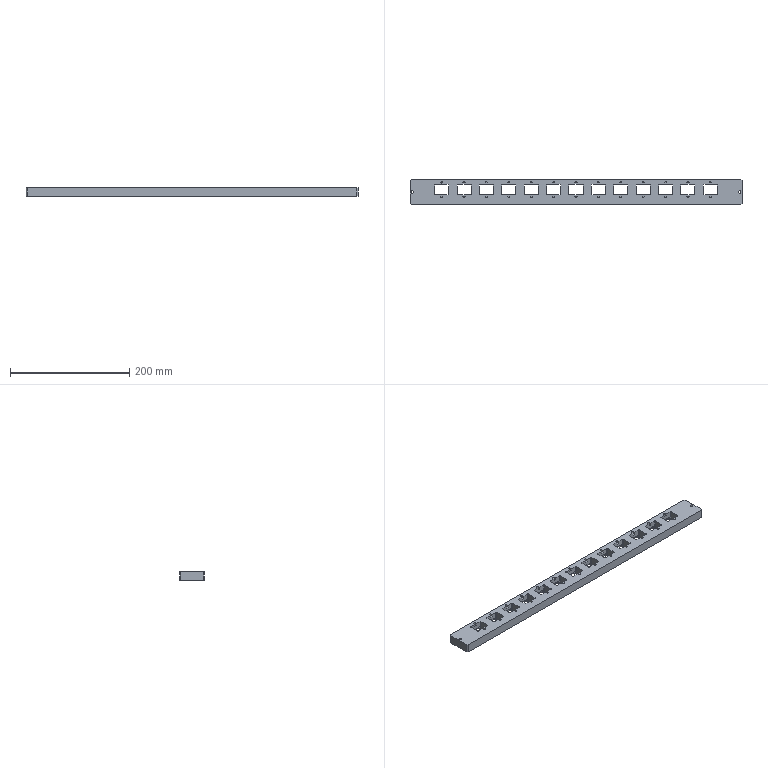NC program | NX | posted with a generic post | part box 556 x 41 x 15 mm
Lines 9014 to 9897 of 144595:
(ZLEVEL_PROFILE_COPY_1_COPY , TOOL : D6JING)
N17990 T06 M6
N17992 G54
N17994 G17 G0 G90 X230.494 Y-0.55 S5000 M3
N17996 G43 Z30. H6
N17998 Z-0.198
N18000 G94 G1 X231.014 Y-1.45 F1000.
N18002 G3 X231.534 Y-1.75 R0.6
N18004 G1 X233.75 F1800.
N18006 Y0.466
N18008 G3 X233.45 Y0.986 R0.6
N18010 G1 X232.55 Y1.506
N18012 G0 X230.494 Y-0.55 Z-0.396
N18014 G1 X231.014 Y-1.45 F1000.
N18016 G3 X231.534 Y-1.75 R0.6
N18018 G1 X233.75 F1800.
N18020 Y0.466
N18022 G3 X233.45 Y0.986 R0.6
N18024 G1 X232.55 Y1.506
N18026 G0 X230.494 Y-0.55 Z-0.594
N18028 G1 X231.014 Y-1.45 F1000.
N18030 G3 X231.534 Y-1.75 R0.6
N18032 G1 X233.75 F1800.
N18034 Y0.466
N18036 G3 X233.45 Y0.986 R0.6
N18038 G1 X232.55 Y1.506
N18040 G0 X230.494 Y-0.55 Z-0.792
N18042 G1 X231.014 Y-1.45 F1000.
N18044 G3 X231.534 Y-1.75 R0.6
N18046 G1 X233.75 F1800.
N18048 Y0.466
N18050 G3 X233.45 Y0.986 R0.6
N18052 G1 X232.55 Y1.506
N18054 G0 X230.494 Y-0.55 Z-0.99
N18056 G1 X231.014 Y-1.45 F1000.
N18058 G3 X231.534 Y-1.75 R0.6
N18060 G1 X233.75 F1800.
N18062 Y0.466
N18064 G3 X233.45 Y0.986 R0.6
N18066 G1 X232.55 Y1.506
N18068 G0 X230.494 Y-0.55 Z-1.188
N18070 G1 X231.014 Y-1.45 F1000.
N18072 G3 X231.534 Y-1.75 R0.6
N18074 G1 X233.75 F1800.
N18076 Y0.466
N18078 G3 X233.45 Y0.986 R0.6
N18080 G1 X232.55 Y1.506
N18082 G0 X230.494 Y-0.55 Z-1.386
N18084 G1 X231.014 Y-1.45 F1000.
N18086 G3 X231.534 Y-1.75 R0.6
N18088 G1 X233.75 F1800.
N18090 Y0.466
N18092 G3 X233.45 Y0.986 R0.6
N18094 G1 X232.55 Y1.506
N18096 G0 X230.494 Y-0.55 Z-1.584
N18098 G1 X231.014 Y-1.45 F1000.
N18100 G3 X231.534 Y-1.75 R0.6
N18102 G1 X233.75 F1800.
N18104 Y0.466
N18106 G3 X233.45 Y0.986 R0.6
N18108 G1 X232.55 Y1.506
N18110 G0 X230.494 Y-0.55 Z-1.782
N18112 G1 X231.014 Y-1.45 F1000.
N18114 G3 X231.534 Y-1.75 R0.6
N18116 G1 X233.75 F1800.
N18118 Y0.466
N18120 G3 X233.45 Y0.986 R0.6
N18122 G1 X232.55 Y1.506
N18124 G0 X230.494 Y-0.55 Z-1.98
N18126 G1 X231.014 Y-1.45 F1000.
N18128 G3 X231.534 Y-1.75 R0.6
N18130 G1 X233.75 F1800.
N18132 Y0.466
N18134 G3 X233.45 Y0.986 R0.6
N18136 G1 X232.55 Y1.506
N18138 G0 X230.494 Y-0.55 Z-2.178
N18140 G1 X231.014 Y-1.45 F1000.
N18142 G3 X231.534 Y-1.75 R0.6
N18144 G1 X233.75 F1800.
N18146 Y0.466
N18148 G3 X233.45 Y0.986 R0.6
N18150 G1 X232.55 Y1.506
N18152 G0 X230.494 Y-0.55 Z-2.376
N18154 G1 X231.014 Y-1.45 F1000.
N18156 G3 X231.534 Y-1.75 R0.6
N18158 G1 X233.75 F1800.
N18160 Y0.466
N18162 G3 X233.45 Y0.986 R0.6
N18164 G1 X232.55 Y1.506
N18166 G0 X230.494 Y-0.55 Z-2.574
N18168 G1 X231.014 Y-1.45 F1000.
N18170 G3 X231.534 Y-1.75 R0.6
N18172 G1 X233.75 F1800.
N18174 Y0.466
N18176 G3 X233.45 Y0.986 R0.6
N18178 G1 X232.55 Y1.506
N18180 G0 X230.494 Y-0.55 Z-2.772
N18182 G1 X231.014 Y-1.45 F1000.
N18184 G3 X231.534 Y-1.75 R0.6
N18186 G1 X233.75 F1800.
N18188 Y0.466
N18190 G3 X233.45 Y0.986 R0.6
N18192 G1 X232.55 Y1.506
N18194 G0 X230.494 Y-0.55 Z-2.97
N18196 G1 X231.014 Y-1.45 F1000.
N18198 G3 X231.534 Y-1.75 R0.6
N18200 G1 X233.75 F1800.
N18202 Y0.466
N18204 G3 X233.45 Y0.986 R0.6
N18206 G1 X232.55 Y1.506
N18208 G0 X230.494 Y-0.55 Z-3.168
N18210 G1 X231.014 Y-1.45 F1000.
N18212 G3 X231.534 Y-1.75 R0.6
N18214 G1 X233.75 F1800.
N18216 Y0.466
N18218 G3 X233.45 Y0.986 R0.6
N18220 G1 X232.55 Y1.506
N18222 G0 X230.494 Y-0.55 Z-3.366
N18224 G1 X231.014 Y-1.45 F1000.
N18226 G3 X231.534 Y-1.75 R0.6
N18228 G1 X233.75 F1800.
N18230 Y0.466
N18232 G3 X233.45 Y0.986 R0.6
N18234 G1 X232.55 Y1.506
N18236 G0 X230.494 Y-0.55 Z-3.564
N18238 G1 X231.014 Y-1.45 F1000.
N18240 G3 X231.534 Y-1.75 R0.6
N18242 G1 X233.75 F1800.
N18244 Y0.466
N18246 G3 X233.45 Y0.986 R0.6
N18248 G1 X232.55 Y1.506
N18250 G0 X230.494 Y-0.55 Z-3.762
N18252 G1 X231.014 Y-1.45 F1000.
N18254 G3 X231.534 Y-1.75 R0.6
N18256 G1 X233.75 F1800.
N18258 Y0.466
N18260 G3 X233.45 Y0.986 R0.6
N18262 G1 X232.55 Y1.506
N18264 G0 X230.494 Y-0.55 Z-3.96
N18266 G1 X231.014 Y-1.45 F1000.
N18268 G3 X231.534 Y-1.75 R0.6
N18270 G1 X233.75 F1800.
N18272 Y0.466
N18274 G3 X233.45 Y0.986 R0.6
N18276 G1 X232.55 Y1.506
N18278 G0 X230.494 Y-0.55 Z-4.158
N18280 G1 X231.014 Y-1.45 F1000.
N18282 G3 X231.534 Y-1.75 R0.6
N18284 G1 X233.75 F1800.
N18286 Y0.466
N18288 G3 X233.45 Y0.986 R0.6
N18290 G1 X232.55 Y1.506
N18292 G0 X230.494 Y-0.55 Z-4.356
N18294 G1 X231.014 Y-1.45 F1000.
N18296 G3 X231.534 Y-1.75 R0.6
N18298 G1 X233.75 F1800.
N18300 Y0.466
N18302 G3 X233.45 Y0.986 R0.6
N18304 G1 X232.55 Y1.506
N18306 G0 X230.494 Y-0.55 Z-4.554
N18308 G1 X231.014 Y-1.45 F1000.
N18310 G3 X231.534 Y-1.75 R0.6
N18312 G1 X233.75 F1800.
N18314 Y0.466
N18316 G3 X233.45 Y0.986 R0.6
N18318 G1 X232.55 Y1.506
N18320 G0 X230.494 Y-0.55 Z-4.752
N18322 G1 X231.014 Y-1.45 F1000.
N18324 G3 X231.534 Y-1.75 R0.6
N18326 G1 X233.75 F1800.
N18328 Y0.466
N18330 G3 X233.45 Y0.986 R0.6
N18332 G1 X232.55 Y1.506
N18334 G0 X230.494 Y-0.55 Z-4.95
N18336 G1 X231.014 Y-1.45 F1000.
N18338 G3 X231.534 Y-1.75 R0.6
N18340 G1 X233.75 F1800.
N18342 Y0.466
N18344 G3 X233.45 Y0.986 R0.6
N18346 G1 X232.55 Y1.506
N18348 G0 X230.494 Y-0.55 Z-5.148
N18350 G1 X231.014 Y-1.45 F1000.
N18352 G3 X231.534 Y-1.75 R0.6
N18354 G1 X233.75 F1800.
N18356 Y0.466
N18358 G3 X233.45 Y0.986 R0.6
N18360 G1 X232.55 Y1.506
N18362 G0 X230.494 Y-0.55 Z-5.346
N18364 G1 X231.014 Y-1.45 F1000.
N18366 G3 X231.534 Y-1.75 R0.6
N18368 G1 X233.75 F1800.
N18370 Y0.466
N18372 G3 X233.45 Y0.986 R0.6
N18374 G1 X232.55 Y1.506
N18376 G0 X230.494 Y-0.55 Z-5.544
N18378 G1 X231.014 Y-1.45 F1000.
N18380 G3 X231.534 Y-1.75 R0.6
N18382 G1 X233.75 F1800.
N18384 Y0.466
N18386 G3 X233.45 Y0.986 R0.6
N18388 G1 X232.55 Y1.506
N18390 G0 X230.494 Y-0.55 Z-5.742
N18392 G1 X231.014 Y-1.45 F1000.
N18394 G3 X231.534 Y-1.75 R0.6
N18396 G1 X233.75 F1800.
N18398 Y0.466
N18400 G3 X233.45 Y0.986 R0.6
N18402 G1 X232.55 Y1.506
N18404 G0 X230.494 Y-0.55 Z-5.94
N18406 G1 X231.014 Y-1.45 F1000.
N18408 G3 X231.534 Y-1.75 R0.6
N18410 G1 X233.75 F1800.
N18412 Y0.466
N18414 G3 X233.45 Y0.986 R0.6
N18416 G1 X232.55 Y1.506
N18418 G0 X230.494 Y-0.55 Z-6.138
N18420 G1 X231.014 Y-1.45 F1000.
N18422 G3 X231.534 Y-1.75 R0.6
N18424 G1 X233.75 F1800.
N18426 Y0.466
N18428 G3 X233.45 Y0.986 R0.6
N18430 G1 X232.55 Y1.506
N18432 G0 X230.494 Y-0.55 Z-6.336
N18434 G1 X231.014 Y-1.45 F1000.
N18436 G3 X231.534 Y-1.75 R0.6
N18438 G1 X233.75 F1800.
N18440 Y0.466
N18442 G3 X233.45 Y0.986 R0.6
N18444 G1 X232.55 Y1.506
N18446 G0 X230.494 Y-0.55 Z-6.534
N18448 G1 X231.014 Y-1.45 F1000.
N18450 G3 X231.534 Y-1.75 R0.6
N18452 G1 X233.75 F1800.
N18454 Y0.466
N18456 G3 X233.45 Y0.986 R0.6
N18458 G1 X232.55 Y1.506
N18460 G0 X230.494 Y-0.55 Z-6.732
N18462 G1 X231.014 Y-1.45 F1000.
N18464 G3 X231.534 Y-1.75 R0.6
N18466 G1 X233.75 F1800.
N18468 Y0.466
N18470 G3 X233.45 Y0.986 R0.6
N18472 G1 X232.55 Y1.506
N18474 G0 X230.494 Y-0.55 Z-6.93
N18476 G1 X231.014 Y-1.45 F1000.
N18478 G3 X231.534 Y-1.75 R0.6
N18480 G1 X233.75 F1800.
N18482 Y0.466
N18484 G3 X233.45 Y0.986 R0.6
N18486 G1 X232.55 Y1.506
N18488 G0 X230.494 Y-0.55 Z-7.128
N18490 G1 X231.014 Y-1.45 F1000.
N18492 G3 X231.534 Y-1.75 R0.6
N18494 G1 X233.75 F1800.
N18496 Y0.466
N18498 G3 X233.45 Y0.986 R0.6
N18500 G1 X232.55 Y1.506
N18502 G0 X230.494 Y-0.55 Z-7.326
N18504 G1 X231.014 Y-1.45 F1000.
N18506 G3 X231.534 Y-1.75 R0.6
N18508 G1 X233.75 F1800.
N18510 Y0.466
N18512 G3 X233.45 Y0.986 R0.6
N18514 G1 X232.55 Y1.506
N18516 G0 X230.494 Y-0.55 Z-7.524
N18518 G1 X231.014 Y-1.45 F1000.
N18520 G3 X231.534 Y-1.75 R0.6
N18522 G1 X233.75 F1800.
N18524 Y0.466
N18526 G3 X233.45 Y0.986 R0.6
N18528 G1 X232.55 Y1.506
N18530 G0 X230.494 Y-0.55 Z-7.722
N18532 G1 X231.014 Y-1.45 F1000.
N18534 G3 X231.534 Y-1.75 R0.6
N18536 G1 X233.75 F1800.
N18538 Y0.466
N18540 G3 X233.45 Y0.986 R0.6
N18542 G1 X232.55 Y1.506
N18544 G0 X230.494 Y-0.55 Z-7.92
N18546 G1 X231.014 Y-1.45 F1000.
N18548 G3 X231.534 Y-1.75 R0.6
N18550 G1 X233.75 F1800.
N18552 Y0.466
N18554 G3 X233.45 Y0.986 R0.6
N18556 G1 X232.55 Y1.506
N18558 G0 X230.494 Y-0.55 Z-8.118
N18560 G1 X231.014 Y-1.45 F1000.
N18562 G3 X231.534 Y-1.75 R0.6
N18564 G1 X233.75 F1800.
N18566 Y0.466
N18568 G3 X233.45 Y0.986 R0.6
N18570 G1 X232.55 Y1.506
N18572 G0 X230.494 Y-0.55 Z-8.316
N18574 G1 X231.014 Y-1.45 F1000.
N18576 G3 X231.534 Y-1.75 R0.6
N18578 G1 X233.75 F1800.
N18580 Y0.466
N18582 G3 X233.45 Y0.986 R0.6
N18584 G1 X232.55 Y1.506
N18586 G0 X230.494 Y-0.55 Z-8.514
N18588 G1 X231.014 Y-1.45 F1000.
N18590 G3 X231.534 Y-1.75 R0.6
N18592 G1 X233.75 F1800.
N18594 Y0.466
N18596 G3 X233.45 Y0.986 R0.6
N18598 G1 X232.55 Y1.506
N18600 G0 X230.494 Y-0.55 Z-8.712
N18602 G1 X231.014 Y-1.45 F1000.
N18604 G3 X231.534 Y-1.75 R0.6
N18606 G1 X233.75 F1800.
N18608 Y0.466
N18610 G3 X233.45 Y0.986 R0.6
N18612 G1 X232.55 Y1.506
N18614 G0 X230.494 Y-0.55 Z-8.91
N18616 G1 X231.014 Y-1.45 F1000.
N18618 G3 X231.534 Y-1.75 R0.6
N18620 G1 X233.75 F1800.
N18622 Y0.466
N18624 G3 X233.45 Y0.986 R0.6
N18626 G1 X232.55 Y1.506
N18628 G0 X230.494 Y-0.55 Z-9.108
N18630 G1 X231.014 Y-1.45 F1000.
N18632 G3 X231.534 Y-1.75 R0.6
N18634 G1 X233.75 F1800.
N18636 Y0.466
N18638 G3 X233.45 Y0.986 R0.6
N18640 G1 X232.55 Y1.506
N18642 G0 X230.494 Y-0.55 Z-9.306
N18644 G1 X231.014 Y-1.45 F1000.
N18646 G3 X231.534 Y-1.75 R0.6
N18648 G1 X233.75 F1800.
N18650 Y0.466
N18652 G3 X233.45 Y0.986 R0.6
N18654 G1 X232.55 Y1.506
N18656 G0 X230.494 Y-0.55 Z-9.504
N18658 G1 X231.014 Y-1.45 F1000.
N18660 G3 X231.534 Y-1.75 R0.6
N18662 G1 X233.75 F1800.
N18664 Y0.466
N18666 G3 X233.45 Y0.986 R0.6
N18668 G1 X232.55 Y1.506
N18670 G0 X230.494 Y-0.55 Z-9.702
N18672 G1 X231.014 Y-1.45 F1000.
N18674 G3 X231.534 Y-1.75 R0.6
N18676 G1 X233.75 F1800.
N18678 Y0.466
N18680 G3 X233.45 Y0.986 R0.6
N18682 G1 X232.55 Y1.506
N18684 G0 X230.494 Y-0.55 Z-9.9
N18686 G1 X231.014 Y-1.45 F1000.
N18688 G3 X231.534 Y-1.75 R0.6
N18690 G1 X233.75 F1800.
N18692 Y0.466
N18694 G3 X233.45 Y0.986 R0.6
N18696 G1 X232.55 Y1.506
N18698 G0 X230.494 Y-0.55 Z-10.098
N18700 G1 X231.014 Y-1.45 F1000.
N18702 G3 X231.534 Y-1.75 R0.6
N18704 G1 X233.75 F1800.
N18706 Y0.466
N18708 G3 X233.45 Y0.986 R0.6
N18710 G1 X232.55 Y1.506
N18712 G0 X230.494 Y-0.55 Z-10.296
N18714 G1 X231.014 Y-1.45 F1000.
N18716 G3 X231.534 Y-1.75 R0.6
N18718 G1 X233.75 F1800.
N18720 Y0.466
N18722 G3 X233.45 Y0.986 R0.6
N18724 G1 X232.55 Y1.506
N18726 G0 X230.494 Y-0.55 Z-10.494
N18728 G1 X231.014 Y-1.45 F1000.
N18730 G3 X231.534 Y-1.75 R0.6
N18732 G1 X233.75 F1800.
N18734 Y0.466
N18736 G3 X233.45 Y0.986 R0.6
N18738 G1 X232.55 Y1.506
N18740 G0 X230.494 Y-0.55 Z-10.692
N18742 G1 X231.014 Y-1.45 F1000.
N18744 G3 X231.534 Y-1.75 R0.6
N18746 G1 X233.75 F1800.
N18748 Y0.466
N18750 G3 X233.45 Y0.986 R0.6
N18752 G1 X232.55 Y1.506
N18754 G0 X230.494 Y-0.55 Z-10.89
N18756 G1 X231.014 Y-1.45 F1000.
N18758 G3 X231.534 Y-1.75 R0.6
N18760 G1 X233.75 F1800.
N18762 Y0.466
N18764 G3 X233.45 Y0.986 R0.6
N18766 G1 X232.55 Y1.506
N18768 G0 X230.494 Y-0.55 Z-11.088
N18770 G1 X231.014 Y-1.45 F1000.
N18772 G3 X231.534 Y-1.75 R0.6
N18774 G1 X233.75 F1800.
N18776 Y0.466
N18778 G3 X233.45 Y0.986 R0.6
N18780 G1 X232.55 Y1.506
N18782 G0 X230.494 Y-0.55 Z-11.286
N18784 G1 X231.014 Y-1.45 F1000.
N18786 G3 X231.534 Y-1.75 R0.6
N18788 G1 X233.75 F1800.
N18790 Y0.466
N18792 G3 X233.45 Y0.986 R0.6
N18794 G1 X232.55 Y1.506
N18796 G0 X230.494 Y-0.55 Z-11.484
N18798 G1 X231.014 Y-1.45 F1000.
N18800 G3 X231.534 Y-1.75 R0.6
N18802 G1 X233.75 F1800.
N18804 Y0.466
N18806 G3 X233.45 Y0.986 R0.6
N18808 G1 X232.55 Y1.506
N18810 G0 X230.494 Y-0.55 Z-11.682
N18812 G1 X231.014 Y-1.45 F1000.
N18814 G3 X231.534 Y-1.75 R0.6
N18816 G1 X233.75 F1800.
N18818 Y0.466
N18820 G3 X233.45 Y0.986 R0.6
N18822 G1 X232.55 Y1.506
N18824 G0 X230.494 Y-0.55 Z-11.88
N18826 G1 X231.014 Y-1.45 F1000.
N18828 G3 X231.534 Y-1.75 R0.6
N18830 G1 X233.75 F1800.
N18832 Y0.466
N18834 G3 X233.45 Y0.986 R0.6
N18836 G1 X232.55 Y1.506
N18838 G0 X230.494 Y-0.55 Z-12.078
N18840 G1 X231.014 Y-1.45 F1000.
N18842 G3 X231.534 Y-1.75 R0.6
N18844 G1 X233.75 F1800.
N18846 Y0.466
N18848 G3 X233.45 Y0.986 R0.6
N18850 G1 X232.55 Y1.506
N18852 G0 X230.494 Y-0.55 Z-12.276
N18854 G1 X231.014 Y-1.45 F1000.
N18856 G3 X231.534 Y-1.75 R0.6
N18858 G1 X233.75 F1800.
N18860 Y0.466
N18862 G3 X233.45 Y0.986 R0.6
N18864 G1 X232.55 Y1.506
N18866 G0 X230.494 Y-0.55 Z-12.474
N18868 G1 X231.014 Y-1.45 F1000.
N18870 G3 X231.534 Y-1.75 R0.6
N18872 G1 X233.75 F1800.
N18874 Y0.466
N18876 G3 X233.45 Y0.986 R0.6
N18878 G1 X232.55 Y1.506
N18880 G0 X230.494 Y-0.55 Z-12.672
N18882 G1 X231.014 Y-1.45 F1000.
N18884 G3 X231.534 Y-1.75 R0.6
N18886 G1 X233.75 F1800.
N18888 Y0.466
N18890 G3 X233.45 Y0.986 R0.6
N18892 G1 X232.55 Y1.506
N18894 G0 X230.494 Y-0.55 Z-12.87
N18896 G1 X231.014 Y-1.45 F1000.
N18898 G3 X231.534 Y-1.75 R0.6
N18900 G1 X233.75 F1800.
N18902 Y0.466
N18904 G3 X233.45 Y0.986 R0.6
N18906 G1 X232.55 Y1.506
N18908 G0 X230.494 Y-0.55 Z-13.068
N18910 G1 X231.014 Y-1.45 F1000.
N18912 G3 X231.534 Y-1.75 R0.6
N18914 G1 X233.75 F1800.
N18916 Y0.466
N18918 G3 X233.45 Y0.986 R0.6
N18920 G1 X232.55 Y1.506
N18922 G0 X230.494 Y-0.55 Z-13.266
N18924 G1 X231.014 Y-1.45 F1000.
N18926 G3 X231.534 Y-1.75 R0.6
N18928 G1 X233.75 F1800.
N18930 Y0.466
N18932 G3 X233.45 Y0.986 R0.6
N18934 G1 X232.55 Y1.506
N18936 G0 X230.494 Y-0.55 Z-13.464
N18938 G1 X231.014 Y-1.45 F1000.
N18940 G3 X231.534 Y-1.75 R0.6
N18942 G1 X233.75 F1800.
N18944 Y0.466
N18946 G3 X233.45 Y0.986 R0.6
N18948 G1 X232.55 Y1.506
N18950 G0 X230.494 Y-0.55 Z-13.662
N18952 G1 X231.014 Y-1.45 F1000.
N18954 G3 X231.534 Y-1.75 R0.6
N18956 G1 X233.75 F1800.
N18958 Y0.466
N18960 G3 X233.45 Y0.986 R0.6
N18962 G1 X232.55 Y1.506
N18964 G0 X230.494 Y-0.55 Z-13.86
N18966 G1 X231.014 Y-1.45 F1000.
N18968 G3 X231.534 Y-1.75 R0.6
N18970 G1 X233.75 F1800.
N18972 Y0.466
N18974 G3 X233.45 Y0.986 R0.6
N18976 G1 X232.55 Y1.506
N18978 G0 X230.494 Y-0.55 Z-14.058
N18980 G1 X231.014 Y-1.45 F1000.
N18982 G3 X231.534 Y-1.75 R0.6
N18984 G1 X233.75 F1800.
N18986 Y0.466
N18988 G3 X233.45 Y0.986 R0.6
N18990 G1 X232.55 Y1.506
N18992 G0 X230.494 Y-0.55 Z-14.256
N18994 G1 X231.014 Y-1.45 F1000.
N18996 G3 X231.534 Y-1.75 R0.6
N18998 G1 X233.75 F1800.
N19000 Y0.466
N19002 G3 X233.45 Y0.986 R0.6
N19004 G1 X232.55 Y1.506
N19006 G0 X230.494 Y-0.55 Z-14.454
N19008 G1 X231.014 Y-1.45 F1000.
N19010 G3 X231.534 Y-1.75 R0.6
N19012 G1 X233.75 F1800.
N19014 Y0.466
N19016 G3 X233.45 Y0.986 R0.6
N19018 G1 X232.55 Y1.506
N19020 G0 X230.494 Y-0.55 Z-14.652
N19022 G1 X231.014 Y-1.45 F1000.
N19024 G3 X231.534 Y-1.75 R0.6
N19026 G1 X233.75 F1800.
N19028 Y0.466
N19030 G3 X233.45 Y0.986 R0.6
N19032 G1 X232.55 Y1.506
N19034 G0 X230.495 Y-0.55 Z-14.85
N19036 G1 X231.015 Y-1.45 F1000.
N19038 G3 X231.534 Y-1.75 R0.6
N19040 G1 X233.75 F1800.
N19042 Y0.466
N19044 G3 X233.45 Y0.986 R0.6
N19046 G1 X232.55 Y1.506
N19048 G0 Z30.
N19050 Y6.494
N19052 Z-0.198
N19054 G1 X233.45 Y7.014 F1000.
N19056 G3 X233.75 Y7.534 R0.6
N19058 G1 Y9.75 F1800.
N19060 X231.534
N19062 G3 X231.014 Y9.45 R0.6
N19064 G1 X230.494 Y8.55
N19066 G0 X232.55 Y6.494 Z-0.396
N19068 G1 X233.45 Y7.014 F1000.
N19070 G3 X233.75 Y7.534 R0.6
N19072 G1 Y9.75 F1800.
N19074 X231.534
N19076 G3 X231.014 Y9.45 R0.6
N19078 G1 X230.494 Y8.55
N19080 G0 X232.55 Y6.494 Z-0.594
N19082 G1 X233.45 Y7.014 F1000.
N19084 G3 X233.75 Y7.534 R0.6
N19086 G1 Y9.75 F1800.
N19088 X231.534
N19090 G3 X231.014 Y9.45 R0.6
N19092 G1 X230.494 Y8.55
N19094 G0 X232.55 Y6.494 Z-0.792
N19096 G1 X233.45 Y7.014 F1000.
N19098 G3 X233.75 Y7.534 R0.6
N19100 G1 Y9.75 F1800.
N19102 X231.534
N19104 G3 X231.014 Y9.45 R0.6
N19106 G1 X230.494 Y8.55
N19108 G0 X232.55 Y6.494 Z-0.99
N19110 G1 X233.45 Y7.014 F1000.
N19112 G3 X233.75 Y7.534 R0.6
N19114 G1 Y9.75 F1800.
N19116 X231.534
N19118 G3 X231.014 Y9.45 R0.6
N19120 G1 X230.494 Y8.55
N19122 G0 X232.55 Y6.494 Z-1.188
N19124 G1 X233.45 Y7.014 F1000.
N19126 G3 X233.75 Y7.534 R0.6
N19128 G1 Y9.75 F1800.
N19130 X231.534
N19132 G3 X231.014 Y9.45 R0.6
N19134 G1 X230.494 Y8.55
N19136 G0 X232.55 Y6.494 Z-1.386
N19138 G1 X233.45 Y7.014 F1000.
N19140 G3 X233.75 Y7.534 R0.6
N19142 G1 Y9.75 F1800.
N19144 X231.534
N19146 G3 X231.014 Y9.45 R0.6
N19148 G1 X230.494 Y8.55
N19150 G0 X232.55 Y6.494 Z-1.584
N19152 G1 X233.45 Y7.014 F1000.
N19154 G3 X233.75 Y7.534 R0.6
N19156 G1 Y9.75 F1800.
N19158 X231.534
N19160 G3 X231.014 Y9.45 R0.6
N19162 G1 X230.494 Y8.55
N19164 G0 X232.55 Y6.494 Z-1.782
N19166 G1 X233.45 Y7.014 F1000.
N19168 G3 X233.75 Y7.534 R0.6
N19170 G1 Y9.75 F1800.
N19172 X231.534
N19174 G3 X231.014 Y9.45 R0.6
N19176 G1 X230.494 Y8.55
N19178 G0 X232.55 Y6.494 Z-1.98
N19180 G1 X233.45 Y7.014 F1000.
N19182 G3 X233.75 Y7.534 R0.6
N19184 G1 Y9.75 F1800.
N19186 X231.534
N19188 G3 X231.014 Y9.45 R0.6
N19190 G1 X230.494 Y8.55
N19192 G0 X232.55 Y6.494 Z-2.178
N19194 G1 X233.45 Y7.014 F1000.
N19196 G3 X233.75 Y7.534 R0.6
N19198 G1 Y9.75 F1800.
N19200 X231.534
N19202 G3 X231.014 Y9.45 R0.6
N19204 G1 X230.494 Y8.55
N19206 G0 X232.55 Y6.494 Z-2.376
N19208 G1 X233.45 Y7.014 F1000.
N19210 G3 X233.75 Y7.534 R0.6
N19212 G1 Y9.75 F1800.
N19214 X231.534
N19216 G3 X231.014 Y9.45 R0.6
N19218 G1 X230.494 Y8.55
N19220 G0 X232.55 Y6.494 Z-2.574
N19222 G1 X233.45 Y7.014 F1000.
N19224 G3 X233.75 Y7.534 R0.6
N19226 G1 Y9.75 F1800.
N19228 X231.534
N19230 G3 X231.014 Y9.45 R0.6
N19232 G1 X230.494 Y8.55
N19234 G0 X232.55 Y6.494 Z-2.772
N19236 G1 X233.45 Y7.014 F1000.
N19238 G3 X233.75 Y7.534 R0.6
N19240 G1 Y9.75 F1800.
N19242 X231.534
N19244 G3 X231.014 Y9.45 R0.6
N19246 G1 X230.494 Y8.55
N19248 G0 X232.55 Y6.494 Z-2.97
N19250 G1 X233.45 Y7.014 F1000.
N19252 G3 X233.75 Y7.534 R0.6
N19254 G1 Y9.75 F1800.
N19256 X231.534
N19258 G3 X231.014 Y9.45 R0.6
N19260 G1 X230.494 Y8.55
N19262 G0 X232.55 Y6.494 Z-3.168
N19264 G1 X233.45 Y7.014 F1000.
N19266 G3 X233.75 Y7.534 R0.6
N19268 G1 Y9.75 F1800.
N19270 X231.534
N19272 G3 X231.014 Y9.45 R0.6
N19274 G1 X230.494 Y8.55
N19276 G0 X232.55 Y6.494 Z-3.366
N19278 G1 X233.45 Y7.014 F1000.
N19280 G3 X233.75 Y7.534 R0.6
N19282 G1 Y9.75 F1800.
N19284 X231.534
N19286 G3 X231.014 Y9.45 R0.6
N19288 G1 X230.494 Y8.55
N19290 G0 X232.55 Y6.494 Z-3.564
N19292 G1 X233.45 Y7.014 F1000.
N19294 G3 X233.75 Y7.534 R0.6
N19296 G1 Y9.75 F1800.
N19298 X231.534
N19300 G3 X231.014 Y9.45 R0.6
N19302 G1 X230.494 Y8.55
N19304 G0 X232.55 Y6.494 Z-3.762
N19306 G1 X233.45 Y7.014 F1000.
N19308 G3 X233.75 Y7.534 R0.6
N19310 G1 Y9.75 F1800.
N19312 X231.534
N19314 G3 X231.014 Y9.45 R0.6
N19316 G1 X230.494 Y8.55
N19318 G0 X232.55 Y6.494 Z-3.96
N19320 G1 X233.45 Y7.014 F1000.
N19322 G3 X233.75 Y7.534 R0.6
N19324 G1 Y9.75 F1800.
N19326 X231.534
N19328 G3 X231.014 Y9.45 R0.6
N19330 G1 X230.494 Y8.55
N19332 G0 X232.55 Y6.494 Z-4.158
N19334 G1 X233.45 Y7.014 F1000.
N19336 G3 X233.75 Y7.534 R0.6
N19338 G1 Y9.75 F1800.
N19340 X231.534
N19342 G3 X231.014 Y9.45 R0.6
N19344 G1 X230.494 Y8.55
N19346 G0 X232.55 Y6.494 Z-4.356
N19348 G1 X233.45 Y7.014 F1000.
N19350 G3 X233.75 Y7.534 R0.6
N19352 G1 Y9.75 F1800.
N19354 X231.534
N19356 G3 X231.014 Y9.45 R0.6
N19358 G1 X230.494 Y8.55
N19360 G0 X232.55 Y6.494 Z-4.554
N19362 G1 X233.45 Y7.014 F1000.
N19364 G3 X233.75 Y7.534 R0.6
N19366 G1 Y9.75 F1800.
N19368 X231.534
N19370 G3 X231.014 Y9.45 R0.6
N19372 G1 X230.494 Y8.55
N19374 G0 X232.55 Y6.494 Z-4.752
N19376 G1 X233.45 Y7.014 F1000.
N19378 G3 X233.75 Y7.534 R0.6
N19380 G1 Y9.75 F1800.
N19382 X231.534
N19384 G3 X231.014 Y9.45 R0.6
N19386 G1 X230.494 Y8.55
N19388 G0 X232.55 Y6.494 Z-4.95
N19390 G1 X233.45 Y7.014 F1000.
N19392 G3 X233.75 Y7.534 R0.6
N19394 G1 Y9.75 F1800.
N19396 X231.534
N19398 G3 X231.014 Y9.45 R0.6
N19400 G1 X230.494 Y8.55
N19402 G0 X232.55 Y6.494 Z-5.148
N19404 G1 X233.45 Y7.014 F1000.
N19406 G3 X233.75 Y7.534 R0.6
N19408 G1 Y9.75 F1800.
N19410 X231.534
N19412 G3 X231.014 Y9.45 R0.6
N19414 G1 X230.494 Y8.55
N19416 G0 X232.55 Y6.494 Z-5.346
N19418 G1 X233.45 Y7.014 F1000.
N19420 G3 X233.75 Y7.534 R0.6
N19422 G1 Y9.75 F1800.
N19424 X231.534
N19426 G3 X231.014 Y9.45 R0.6
N19428 G1 X230.494 Y8.55
N19430 G0 X232.55 Y6.494 Z-5.544
N19432 G1 X233.45 Y7.014 F1000.
N19434 G3 X233.75 Y7.534 R0.6
N19436 G1 Y9.75 F1800.
N19438 X231.534
N19440 G3 X231.014 Y9.45 R0.6
N19442 G1 X230.494 Y8.55
N19444 G0 X232.55 Y6.494 Z-5.742
N19446 G1 X233.45 Y7.014 F1000.
N19448 G3 X233.75 Y7.534 R0.6
N19450 G1 Y9.75 F1800.
N19452 X231.534
N19454 G3 X231.014 Y9.45 R0.6
N19456 G1 X230.494 Y8.55
N19458 G0 X232.55 Y6.494 Z-5.94
N19460 G1 X233.45 Y7.014 F1000.
N19462 G3 X233.75 Y7.534 R0.6
N19464 G1 Y9.75 F1800.
N19466 X231.534
N19468 G3 X231.014 Y9.45 R0.6
N19470 G1 X230.494 Y8.55
N19472 G0 X232.55 Y6.494 Z-6.138
N19474 G1 X233.45 Y7.014 F1000.
N19476 G3 X233.75 Y7.534 R0.6
N19478 G1 Y9.75 F1800.
N19480 X231.534
N19482 G3 X231.014 Y9.45 R0.6
N19484 G1 X230.494 Y8.55
N19486 G0 X232.55 Y6.494 Z-6.336
N19488 G1 X233.45 Y7.014 F1000.
N19490 G3 X233.75 Y7.534 R0.6
N19492 G1 Y9.75 F1800.
N19494 X231.534
N19496 G3 X231.014 Y9.45 R0.6
N19498 G1 X230.494 Y8.55
N19500 G0 X232.55 Y6.494 Z-6.534
N19502 G1 X233.45 Y7.014 F1000.
N19504 G3 X233.75 Y7.534 R0.6
N19506 G1 Y9.75 F1800.
N19508 X231.534
N19510 G3 X231.014 Y9.45 R0.6
N19512 G1 X230.494 Y8.55
N19514 G0 X232.55 Y6.494 Z-6.732
N19516 G1 X233.45 Y7.014 F1000.
N19518 G3 X233.75 Y7.534 R0.6
N19520 G1 Y9.75 F1800.
N19522 X231.534
N19524 G3 X231.014 Y9.45 R0.6
N19526 G1 X230.494 Y8.55
N19528 G0 X232.55 Y6.494 Z-6.93
N19530 G1 X233.45 Y7.014 F1000.
N19532 G3 X233.75 Y7.534 R0.6
N19534 G1 Y9.75 F1800.
N19536 X231.534
N19538 G3 X231.014 Y9.45 R0.6
N19540 G1 X230.494 Y8.55
N19542 G0 X232.55 Y6.494 Z-7.128
N19544 G1 X233.45 Y7.014 F1000.
N19546 G3 X233.75 Y7.534 R0.6
N19548 G1 Y9.75 F1800.
N19550 X231.534
N19552 G3 X231.014 Y9.45 R0.6
N19554 G1 X230.494 Y8.55
N19556 G0 X232.55 Y6.494 Z-7.326
N19558 G1 X233.45 Y7.014 F1000.
N19560 G3 X233.75 Y7.534 R0.6
N19562 G1 Y9.75 F1800.
N19564 X231.534
N19566 G3 X231.014 Y9.45 R0.6
N19568 G1 X230.494 Y8.55
N19570 G0 X232.55 Y6.494 Z-7.524
N19572 G1 X233.45 Y7.014 F1000.
N19574 G3 X233.75 Y7.534 R0.6
N19576 G1 Y9.75 F1800.
N19578 X231.534
N19580 G3 X231.014 Y9.45 R0.6
N19582 G1 X230.494 Y8.55
N19584 G0 X232.55 Y6.494 Z-7.722
N19586 G1 X233.45 Y7.014 F1000.
N19588 G3 X233.75 Y7.534 R0.6
N19590 G1 Y9.75 F1800.
N19592 X231.534
N19594 G3 X231.014 Y9.45 R0.6
N19596 G1 X230.494 Y8.55
N19598 G0 X232.55 Y6.494 Z-7.92
N19600 G1 X233.45 Y7.014 F1000.
N19602 G3 X233.75 Y7.534 R0.6
N19604 G1 Y9.75 F1800.
N19606 X231.534
N19608 G3 X231.014 Y9.45 R0.6
N19610 G1 X230.494 Y8.55
N19612 G0 X232.55 Y6.494 Z-8.118
N19614 G1 X233.45 Y7.014 F1000.
N19616 G3 X233.75 Y7.534 R0.6
N19618 G1 Y9.75 F1800.
N19620 X231.534
N19622 G3 X231.014 Y9.45 R0.6
N19624 G1 X230.494 Y8.55
N19626 G0 X232.55 Y6.494 Z-8.316
N19628 G1 X233.45 Y7.014 F1000.
N19630 G3 X233.75 Y7.534 R0.6
N19632 G1 Y9.75 F1800.
N19634 X231.534
N19636 G3 X231.014 Y9.45 R0.6
N19638 G1 X230.494 Y8.55
N19640 G0 X232.55 Y6.494 Z-8.514
N19642 G1 X233.45 Y7.014 F1000.
N19644 G3 X233.75 Y7.534 R0.6
N19646 G1 Y9.75 F1800.
N19648 X231.534
N19650 G3 X231.014 Y9.45 R0.6
N19652 G1 X230.494 Y8.55
N19654 G0 X232.55 Y6.494 Z-8.712
N19656 G1 X233.45 Y7.014 F1000.
N19658 G3 X233.75 Y7.534 R0.6
N19660 G1 Y9.75 F1800.
N19662 X231.534
N19664 G3 X231.014 Y9.45 R0.6
N19666 G1 X230.494 Y8.55
N19668 G0 X232.55 Y6.494 Z-8.91
N19670 G1 X233.45 Y7.014 F1000.
N19672 G3 X233.75 Y7.534 R0.6
N19674 G1 Y9.75 F1800.
N19676 X231.534
N19678 G3 X231.014 Y9.45 R0.6
N19680 G1 X230.494 Y8.55
N19682 G0 X232.55 Y6.494 Z-9.108
N19684 G1 X233.45 Y7.014 F1000.
N19686 G3 X233.75 Y7.534 R0.6
N19688 G1 Y9.75 F1800.
N19690 X231.534
N19692 G3 X231.014 Y9.45 R0.6
N19694 G1 X230.494 Y8.55
N19696 G0 X232.55 Y6.494 Z-9.306
N19698 G1 X233.45 Y7.014 F1000.
N19700 G3 X233.75 Y7.534 R0.6
N19702 G1 Y9.75 F1800.
N19704 X231.534
N19706 G3 X231.014 Y9.45 R0.6
N19708 G1 X230.494 Y8.55
N19710 G0 X232.55 Y6.494 Z-9.504
N19712 G1 X233.45 Y7.014 F1000.
N19714 G3 X233.75 Y7.534 R0.6
N19716 G1 Y9.75 F1800.
N19718 X231.534
N19720 G3 X231.014 Y9.45 R0.6
N19722 G1 X230.494 Y8.55
N19724 G0 X232.55 Y6.494 Z-9.702
N19726 G1 X233.45 Y7.014 F1000.
N19728 G3 X233.75 Y7.534 R0.6
N19730 G1 Y9.75 F1800.
N19732 X231.534
N19734 G3 X231.014 Y9.45 R0.6
N19736 G1 X230.494 Y8.55
N19738 G0 X232.55 Y6.494 Z-9.9
N19740 G1 X233.45 Y7.014 F1000.
N19742 G3 X233.75 Y7.534 R0.6
N19744 G1 Y9.75 F1800.
N19746 X231.534
N19748 G3 X231.014 Y9.45 R0.6
N19750 G1 X230.494 Y8.55